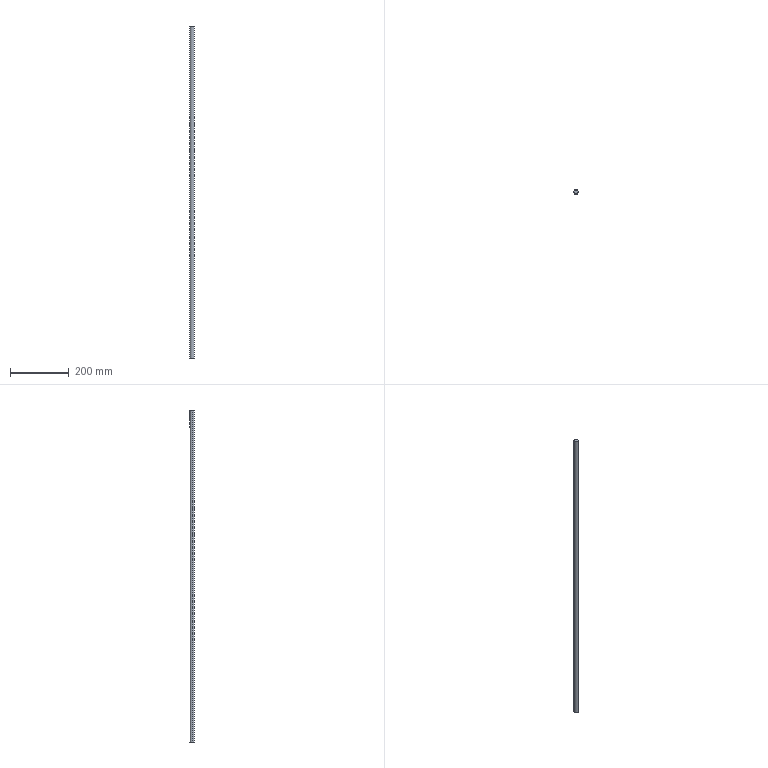Part | SolidWorks | features ICE 3, Extrusion 1 | 1 solid | 14 faces | box 15 x 15 x 1130 mm | volume 199245 mm3 | plane 8 | cylinder 6 | commonest cylinder face diameters 5 x4 15 x2
STEP:
#1=CARTESIAN_POINT('',(0.,7.5,1107.5));
#2=VERTEX_POINT('',#1);
#3=CARTESIAN_POINT('',(2.5,7.071,1110.));
#4=VERTEX_POINT('',#3);
#5=CARTESIAN_POINT('',(0.,7.5,1107.5));
#6=CARTESIAN_POINT('',(0.1643,7.5,1107.5));
#7=CARTESIAN_POINT('',(0.3311,7.494,1107.517));
#8=CARTESIAN_POINT('',(0.6524,7.473,1107.581));
#9=CARTESIAN_POINT('',(0.8088,7.458,1107.629));
#10=CARTESIAN_POINT('',(1.113,7.419,1107.755));
#11=CARTESIAN_POINT('',(1.257,7.395,1107.833));
#12=CARTESIAN_POINT('',(1.526,7.344,1108.013));
#13=CARTESIAN_POINT('',(1.653,7.316,1108.118));
#14=CARTESIAN_POINT('',(1.883,7.261,1108.348));
#15=CARTESIAN_POINT('',(1.986,7.233,1108.473));
#16=CARTESIAN_POINT('',(2.167,7.181,1108.742));
#17=CARTESIAN_POINT('',(2.245,7.156,1108.888));
#18=CARTESIAN_POINT('',(2.37,7.116,1109.189));
#19=CARTESIAN_POINT('',(2.418,7.1,1109.344));
#20=CARTESIAN_POINT('',(2.483,7.077,1109.668));
#21=CARTESIAN_POINT('',(2.5,7.071,1109.834));
#22=CARTESIAN_POINT('',(2.5,7.071,1110.));
#23=B_SPLINE_CURVE_WITH_KNOTS('',3,(#5,#6,#7,#8,#9,#10,#11,#12,#13,#14,#15,#16,#17,#18,#19,#20,#21,#22),.UNSPECIFIED.,.F.,.F.,(4,2,2,2,2,2,2,2,4),(0.003937,0.004429,0.004921,0.005412,0.005904,0.006395,0.006887,0.007378,0.00787),.UNSPECIFIED.);
#24=EDGE_CURVE('',#2,#4,#23,.T.);
#25=ORIENTED_EDGE('',*,*,#24,.F.);
#26=CARTESIAN_POINT('',(0.,4.5,1107.5));
#27=VERTEX_POINT('',#26);
#28=CARTESIAN_POINT('',(0.,7.501,1107.5));
#29=DIRECTION('',(0.,-1.,0.));
#30=VECTOR('',#29,1000.);
#31=LINE('',#28,#30);
#32=EDGE_CURVE('',#2,#27,#31,.T.);
#33=ORIENTED_EDGE('',*,*,#32,.T.);
#34=CARTESIAN_POINT('',(2.5,4.5,1110.));
#35=VERTEX_POINT('',#34);
#36=CARTESIAN_POINT('',(0.,4.5,1110.));
#37=DIRECTION('',(0.,1.,0.));
#38=DIRECTION('',(0.,0.,-1.));
#39=AXIS2_PLACEMENT_3D('',#36,#37,#38);
#40=CIRCLE('',#39,2.5);
#41=EDGE_CURVE('',#35,#27,#40,.T.);
#42=ORIENTED_EDGE('',*,*,#41,.F.);
#43=CARTESIAN_POINT('',(2.5,7.071,1110.));
#44=DIRECTION('',(0.,1.,0.));
#45=VECTOR('',#44,1000.);
#46=LINE('',#43,#45);
#47=EDGE_CURVE('',#35,#4,#46,.T.);
#48=ORIENTED_EDGE('',*,*,#47,.T.);
#49=EDGE_LOOP('',(#25,#33,#42,#48));
#50=FACE_OUTER_BOUND('',#49,.T.);
#51=CARTESIAN_POINT('',(0.,7.501,1110.));
#52=DIRECTION('',(0.,-1.,0.));
#53=DIRECTION('',(0.,0.,-1.));
#54=AXIS2_PLACEMENT_3D('',#51,#52,#53);
#55=CYLINDRICAL_SURFACE('',#54,2.5);
#56=ADVANCED_FACE('',(#50),#55,.F.);
#57=CARTESIAN_POINT('',(-2.5,7.071,1079.079));
#58=VERTEX_POINT('',#57);
#59=CARTESIAN_POINT('',(2.5,7.071,1079.079));
#60=VERTEX_POINT('',#59);
#61=CARTESIAN_POINT('',(-2.5,7.071,1079.079));
#62=CARTESIAN_POINT('',(-2.5,7.071,1079.245));
#63=CARTESIAN_POINT('',(-2.484,7.077,1079.409));
#64=CARTESIAN_POINT('',(-2.419,7.099,1079.73));
#65=CARTESIAN_POINT('',(-2.371,7.116,1079.889));
#66=CARTESIAN_POINT('',(-2.245,7.156,1080.191));
#67=CARTESIAN_POINT('',(-2.168,7.18,1080.334));
#68=CARTESIAN_POINT('',(-1.987,7.233,1080.605));
#69=CARTESIAN_POINT('',(-1.882,7.261,1080.732));
#70=CARTESIAN_POINT('',(-1.539,7.344,1081.075));
#71=CARTESIAN_POINT('',(-1.262,7.399,1081.261));
#72=CARTESIAN_POINT('',(-0.812,7.457,1081.449));
#73=CARTESIAN_POINT('',(-0.6532,7.473,1081.498));
#74=CARTESIAN_POINT('',(-0.33,7.494,1081.563));
#75=CARTESIAN_POINT('',(-0.167,7.5,1081.579));
#76=CARTESIAN_POINT('',(0.1617,7.5,1081.579));
#77=CARTESIAN_POINT('',(0.3287,7.495,1081.563));
#78=CARTESIAN_POINT('',(0.6503,7.473,1081.499));
#79=CARTESIAN_POINT('',(0.8068,7.458,1081.451));
#80=CARTESIAN_POINT('',(1.111,7.419,1081.325));
#81=CARTESIAN_POINT('',(1.255,7.395,1081.247));
#82=CARTESIAN_POINT('',(1.525,7.345,1081.067));
#83=CARTESIAN_POINT('',(1.652,7.317,1080.962));
#84=CARTESIAN_POINT('',(1.882,7.261,1080.732));
#85=CARTESIAN_POINT('',(1.985,7.233,1080.607));
#86=CARTESIAN_POINT('',(2.166,7.181,1080.338));
#87=CARTESIAN_POINT('',(2.245,7.156,1080.192));
#88=CARTESIAN_POINT('',(2.37,7.116,1079.891));
#89=CARTESIAN_POINT('',(2.418,7.1,1079.735));
#90=CARTESIAN_POINT('',(2.483,7.077,1079.412));
#91=CARTESIAN_POINT('',(2.5,7.071,1079.245));
#92=CARTESIAN_POINT('',(2.5,7.071,1079.079));
#93=B_SPLINE_CURVE_WITH_KNOTS('',3,(#61,#62,#63,#64,#65,#66,#67,#68,#69,#70,#71,#72,#73,#74,#75,#76,#77,#78,#79,#80,#81,#82,#83,#84,#85,#86,#87,#88,#89,#90,#91,#92),.UNSPECIFIED.,.F.,.F.,(4,2,2,2,2,2,2,2,2,2,2,2,2,2,2,4),(0.,0.0004919,0.0009837,0.001476,0.001967,0.002951,0.003443,0.003935,0.004427,0.004919,0.00541,0.005902,0.006394,0.006886,0.007378,0.00787),.UNSPECIFIED.);
#94=EDGE_CURVE('',#58,#60,#93,.T.);
#95=ORIENTED_EDGE('',*,*,#94,.F.);
#96=CARTESIAN_POINT('',(-2.5,7.071,1074.079));
#97=VERTEX_POINT('',#96);
#98=CARTESIAN_POINT('',(-2.5,7.071,1130.));
#99=DIRECTION('',(0.,0.,1.));
#100=VECTOR('',#99,1000.);
#101=LINE('',#98,#100);
#102=EDGE_CURVE('',#97,#58,#101,.T.);
#103=ORIENTED_EDGE('',*,*,#102,.F.);
#104=CARTESIAN_POINT('',(2.5,7.071,1074.079));
#105=VERTEX_POINT('',#104);
#106=CARTESIAN_POINT('',(2.5,7.071,1074.079));
#107=CARTESIAN_POINT('',(2.5,7.071,1073.913));
#108=CARTESIAN_POINT('',(2.484,7.077,1073.749));
#109=CARTESIAN_POINT('',(2.419,7.099,1073.428));
#110=CARTESIAN_POINT('',(2.371,7.116,1073.269));
#111=CARTESIAN_POINT('',(2.245,7.156,1072.967));
#112=CARTESIAN_POINT('',(2.168,7.18,1072.824));
#113=CARTESIAN_POINT('',(1.987,7.233,1072.553));
#114=CARTESIAN_POINT('',(1.882,7.261,1072.426));
#115=CARTESIAN_POINT('',(1.539,7.344,1072.083));
#116=CARTESIAN_POINT('',(1.262,7.399,1071.897));
#117=CARTESIAN_POINT('',(0.812,7.457,1071.709));
#118=CARTESIAN_POINT('',(0.6532,7.473,1071.66));
#119=CARTESIAN_POINT('',(0.33,7.494,1071.595));
#120=CARTESIAN_POINT('',(0.167,7.5,1071.579));
#121=CARTESIAN_POINT('',(-0.1617,7.5,1071.579));
#122=CARTESIAN_POINT('',(-0.3287,7.495,1071.595));
#123=CARTESIAN_POINT('',(-0.6503,7.473,1071.66));
#124=CARTESIAN_POINT('',(-0.8068,7.458,1071.707));
#125=CARTESIAN_POINT('',(-1.111,7.419,1071.833));
#126=CARTESIAN_POINT('',(-1.255,7.395,1071.911));
#127=CARTESIAN_POINT('',(-1.525,7.345,1072.091));
#128=CARTESIAN_POINT('',(-1.652,7.317,1072.196));
#129=CARTESIAN_POINT('',(-1.882,7.261,1072.426));
#130=CARTESIAN_POINT('',(-1.985,7.233,1072.551));
#131=CARTESIAN_POINT('',(-2.166,7.181,1072.82));
#132=CARTESIAN_POINT('',(-2.245,7.156,1072.967));
#133=CARTESIAN_POINT('',(-2.37,7.116,1073.267));
#134=CARTESIAN_POINT('',(-2.418,7.1,1073.423));
#135=CARTESIAN_POINT('',(-2.483,7.077,1073.746));
#136=CARTESIAN_POINT('',(-2.5,7.071,1073.913));
#137=CARTESIAN_POINT('',(-2.5,7.071,1074.079));
#138=B_SPLINE_CURVE_WITH_KNOTS('',3,(#106,#107,#108,#109,#110,#111,#112,#113,#114,#115,#116,#117,#118,#119,#120,#121,#122,#123,#124,#125,#126,#127,#128,#129,#130,#131,#132,#133,#134,#135,#136,#137),.UNSPECIFIED.,.F.,.F.,(4,2,2,2,2,2,2,2,2,2,2,2,2,2,2,4),(0.,0.0004919,0.0009837,0.001476,0.001967,0.002951,0.003443,0.003935,0.004427,0.004919,0.00541,0.005902,0.006394,0.006886,0.007378,0.00787),.UNSPECIFIED.);
#139=EDGE_CURVE('',#105,#97,#138,.T.);
#140=ORIENTED_EDGE('',*,*,#139,.F.);
#141=CARTESIAN_POINT('',(2.5,7.071,1130.));
#142=DIRECTION('',(0.,0.,-1.));
#143=VECTOR('',#142,1000.);
#144=LINE('',#141,#143);
#145=EDGE_CURVE('',#60,#105,#144,.T.);
#146=ORIENTED_EDGE('',*,*,#145,.F.);
#147=EDGE_LOOP('',(#95,#103,#140,#146));
#148=FACE_BOUND('',#147,.T.);
#149=CARTESIAN_POINT('',(7.5,0.,1130.));
#150=VERTEX_POINT('',#149);
#151=CARTESIAN_POINT('',(2.5,7.071,1130.));
#152=VERTEX_POINT('',#151);
#153=CARTESIAN_POINT('',(0.,0.,1130.));
#154=DIRECTION('',(0.,0.,1.));
#155=DIRECTION('',(1.,0.,0.));
#156=AXIS2_PLACEMENT_3D('',#153,#154,#155);
#157=CIRCLE('',#156,7.5);
#158=EDGE_CURVE('',#150,#152,#157,.T.);
#159=ORIENTED_EDGE('',*,*,#158,.F.);
#160=CARTESIAN_POINT('',(7.5,0.,0.));
#161=VERTEX_POINT('',#160);
#162=CARTESIAN_POINT('',(7.5,0.,1130.));
#163=DIRECTION('',(0.,0.,-1.));
#164=VECTOR('',#163,1000.);
#165=LINE('',#162,#164);
#166=EDGE_CURVE('',#150,#161,#165,.T.);
#167=ORIENTED_EDGE('',*,*,#166,.T.);
#168=CARTESIAN_POINT('',(-7.5,0.,0.));
#169=VERTEX_POINT('',#168);
#170=CARTESIAN_POINT('',(0.,0.,0.));
#171=DIRECTION('',(0.,0.,1.));
#172=DIRECTION('',(1.,0.,0.));
#173=AXIS2_PLACEMENT_3D('',#170,#171,#172);
#174=CIRCLE('',#173,7.5);
#175=EDGE_CURVE('',#161,#169,#174,.T.);
#176=ORIENTED_EDGE('',*,*,#175,.T.);
#177=CARTESIAN_POINT('',(-7.5,0.,1130.));
#178=VERTEX_POINT('',#177);
#179=CARTESIAN_POINT('',(-7.5,0.,1130.));
#180=DIRECTION('',(0.,0.,-1.));
#181=VECTOR('',#180,1000.);
#182=LINE('',#179,#181);
#183=EDGE_CURVE('',#178,#169,#182,.T.);
#184=ORIENTED_EDGE('',*,*,#183,.F.);
#185=CARTESIAN_POINT('',(-2.5,7.071,1130.));
#186=VERTEX_POINT('',#185);
#187=CARTESIAN_POINT('',(0.,0.,1130.));
#188=DIRECTION('',(0.,0.,1.));
#189=DIRECTION('',(1.,0.,0.));
#190=AXIS2_PLACEMENT_3D('',#187,#188,#189);
#191=CIRCLE('',#190,7.5);
#192=EDGE_CURVE('',#186,#178,#191,.T.);
#193=ORIENTED_EDGE('',*,*,#192,.F.);
#194=CARTESIAN_POINT('',(-2.5,7.071,1110.));
#195=VERTEX_POINT('',#194);
#196=CARTESIAN_POINT('',(-2.5,7.071,1110.));
#197=DIRECTION('',(0.,0.,1.));
#198=VECTOR('',#197,1000.);
#199=LINE('',#196,#198);
#200=EDGE_CURVE('',#195,#186,#199,.T.);
#201=ORIENTED_EDGE('',*,*,#200,.F.);
#202=CARTESIAN_POINT('',(-2.5,7.071,1110.));
#203=CARTESIAN_POINT('',(-2.5,7.071,1109.833));
#204=CARTESIAN_POINT('',(-2.484,7.077,1109.67));
#205=CARTESIAN_POINT('',(-2.419,7.099,1109.349));
#206=CARTESIAN_POINT('',(-2.371,7.116,1109.189));
#207=CARTESIAN_POINT('',(-2.245,7.157,1108.887));
#208=CARTESIAN_POINT('',(-2.168,7.181,1108.744));
#209=CARTESIAN_POINT('',(-1.986,7.233,1108.473));
#210=CARTESIAN_POINT('',(-1.882,7.261,1108.346));
#211=CARTESIAN_POINT('',(-1.538,7.344,1108.003));
#212=CARTESIAN_POINT('',(-1.261,7.399,1107.817));
#213=CARTESIAN_POINT('',(-0.81,7.458,1107.629));
#214=CARTESIAN_POINT('',(-0.6511,7.473,1107.581));
#215=CARTESIAN_POINT('',(-0.3276,7.495,1107.516));
#216=CARTESIAN_POINT('',(-0.1645,7.5,1107.5));
#217=CARTESIAN_POINT('',(0.,7.5,1107.5));
#218=B_SPLINE_CURVE_WITH_KNOTS('',3,(#202,#203,#204,#205,#206,#207,#208,#209,#210,#211,#212,#213,#214,#215,#216,#217),.UNSPECIFIED.,.F.,.F.,(4,2,2,2,2,2,2,4),(0.,0.0004922,0.0009844,0.001477,0.001969,0.002953,0.003445,0.003937),.UNSPECIFIED.);
#219=EDGE_CURVE('',#195,#2,#218,.T.);
#220=ORIENTED_EDGE('',*,*,#219,.T.);
#221=ORIENTED_EDGE('',*,*,#24,.T.);
#222=CARTESIAN_POINT('',(2.5,7.071,1110.));
#223=DIRECTION('',(0.,0.,1.));
#224=VECTOR('',#223,1000.);
#225=LINE('',#222,#224);
#226=EDGE_CURVE('',#4,#152,#225,.T.);
#227=ORIENTED_EDGE('',*,*,#226,.T.);
#228=EDGE_LOOP('',(#159,#167,#176,#184,#193,#201,#220,#221,#227));
#229=FACE_OUTER_BOUND('',#228,.T.);
#230=CARTESIAN_POINT('',(0.,0.,1130.));
#231=DIRECTION('',(0.,0.,-1.));
#232=DIRECTION('',(-1.,0.,0.));
#233=AXIS2_PLACEMENT_3D('',#230,#231,#232);
#234=CYLINDRICAL_SURFACE('',#233,7.5);
#235=ADVANCED_FACE('',(#148,#229),#234,.T.);
#236=ORIENTED_EDGE('',*,*,#166,.F.);
#237=CARTESIAN_POINT('',(0.,0.,1130.));
#238=DIRECTION('',(0.,0.,1.));
#239=DIRECTION('',(1.,0.,0.));
#240=AXIS2_PLACEMENT_3D('',#237,#238,#239);
#241=CIRCLE('',#240,7.5);
#242=EDGE_CURVE('',#178,#150,#241,.T.);
#243=ORIENTED_EDGE('',*,*,#242,.F.);
#244=ORIENTED_EDGE('',*,*,#183,.T.);
#245=CARTESIAN_POINT('',(0.,0.,0.));
#246=DIRECTION('',(0.,0.,1.));
#247=DIRECTION('',(1.,0.,0.));
#248=AXIS2_PLACEMENT_3D('',#245,#246,#247);
#249=CIRCLE('',#248,7.5);
#250=EDGE_CURVE('',#169,#161,#249,.T.);
#251=ORIENTED_EDGE('',*,*,#250,.T.);
#252=EDGE_LOOP('',(#236,#243,#244,#251));
#253=FACE_OUTER_BOUND('',#252,.T.);
#254=CARTESIAN_POINT('',(0.,0.,1130.));
#255=DIRECTION('',(0.,0.,-1.));
#256=DIRECTION('',(-1.,0.,0.));
#257=AXIS2_PLACEMENT_3D('',#254,#255,#256);
#258=CYLINDRICAL_SURFACE('',#257,7.5);
#259=ADVANCED_FACE('',(#253),#258,.T.);
#260=CARTESIAN_POINT('',(2.5,4.5,1130.));
#261=VERTEX_POINT('',#260);
#262=CARTESIAN_POINT('',(2.5,7.071,1130.));
#263=DIRECTION('',(0.,1.,0.));
#264=VECTOR('',#263,1000.);
#265=LINE('',#262,#264);
#266=EDGE_CURVE('',#261,#152,#265,.T.);
#267=ORIENTED_EDGE('',*,*,#266,.F.);
#268=CARTESIAN_POINT('',(-2.5,4.5,1130.));
#269=VERTEX_POINT('',#268);
#270=CARTESIAN_POINT('',(-2.5,4.5,1130.));
#271=DIRECTION('',(1.,0.,0.));
#272=VECTOR('',#271,1000.);
#273=LINE('',#270,#272);
#274=EDGE_CURVE('',#269,#261,#273,.T.);
#275=ORIENTED_EDGE('',*,*,#274,.F.);
#276=CARTESIAN_POINT('',(-2.5,7.071,1130.));
#277=DIRECTION('',(0.,-1.,0.));
#278=VECTOR('',#277,1000.);
#279=LINE('',#276,#278);
#280=EDGE_CURVE('',#186,#269,#279,.T.);
#281=ORIENTED_EDGE('',*,*,#280,.F.);
#282=ORIENTED_EDGE('',*,*,#192,.T.);
#283=ORIENTED_EDGE('',*,*,#242,.T.);
#284=ORIENTED_EDGE('',*,*,#158,.T.);
#285=EDGE_LOOP('',(#267,#275,#281,#282,#283,#284));
#286=FACE_OUTER_BOUND('',#285,.T.);
#287=CARTESIAN_POINT('',(0.,0.,1130.));
#288=DIRECTION('',(0.,0.,1.));
#289=DIRECTION('',(1.,0.,0.));
#290=AXIS2_PLACEMENT_3D('',#287,#288,#289);
#291=PLANE('',#290);
#292=ADVANCED_FACE('',(#286),#291,.T.);
#293=ORIENTED_EDGE('',*,*,#250,.F.);
#294=ORIENTED_EDGE('',*,*,#175,.F.);
#295=EDGE_LOOP('',(#293,#294));
#296=FACE_OUTER_BOUND('',#295,.T.);
#297=CARTESIAN_POINT('',(0.,0.,0.));
#298=DIRECTION('',(0.,0.,1.));
#299=DIRECTION('',(1.,0.,0.));
#300=AXIS2_PLACEMENT_3D('',#297,#298,#299);
#301=PLANE('',#300);
#302=ADVANCED_FACE('',(#296),#301,.F.);
#303=ORIENTED_EDGE('',*,*,#266,.T.);
#304=ORIENTED_EDGE('',*,*,#226,.F.);
#305=ORIENTED_EDGE('',*,*,#47,.F.);
#306=CARTESIAN_POINT('',(2.5,4.5,1110.));
#307=DIRECTION('',(0.,0.,1.));
#308=VECTOR('',#307,1000.);
#309=LINE('',#306,#308);
#310=EDGE_CURVE('',#35,#261,#309,.T.);
#311=ORIENTED_EDGE('',*,*,#310,.T.);
#312=EDGE_LOOP('',(#303,#304,#305,#311));
#313=FACE_OUTER_BOUND('',#312,.T.);
#314=CARTESIAN_POINT('',(2.5,7.071,1110.));
#315=DIRECTION('',(1.,0.,0.));
#316=DIRECTION('',(0.,1.,0.));
#317=AXIS2_PLACEMENT_3D('',#314,#315,#316);
#318=PLANE('',#317);
#319=ADVANCED_FACE('',(#313),#318,.F.);
#320=ORIENTED_EDGE('',*,*,#274,.T.);
#321=ORIENTED_EDGE('',*,*,#310,.F.);
#322=ORIENTED_EDGE('',*,*,#41,.T.);
#323=CARTESIAN_POINT('',(-2.5,4.5,1110.));
#324=VERTEX_POINT('',#323);
#325=CARTESIAN_POINT('',(0.,4.5,1110.));
#326=DIRECTION('',(0.,1.,0.));
#327=DIRECTION('',(0.,0.,-1.));
#328=AXIS2_PLACEMENT_3D('',#325,#326,#327);
#329=CIRCLE('',#328,2.5);
#330=EDGE_CURVE('',#27,#324,#329,.T.);
#331=ORIENTED_EDGE('',*,*,#330,.T.);
#332=CARTESIAN_POINT('',(-2.5,4.5,1110.));
#333=DIRECTION('',(0.,0.,1.));
#334=VECTOR('',#333,1000.);
#335=LINE('',#332,#334);
#336=EDGE_CURVE('',#324,#269,#335,.T.);
#337=ORIENTED_EDGE('',*,*,#336,.T.);
#338=EDGE_LOOP('',(#320,#321,#322,#331,#337));
#339=FACE_OUTER_BOUND('',#338,.T.);
#340=CARTESIAN_POINT('',(-2.5,4.5,1110.));
#341=DIRECTION('',(0.,-1.,0.));
#342=DIRECTION('',(1.,0.,0.));
#343=AXIS2_PLACEMENT_3D('',#340,#341,#342);
#344=PLANE('',#343);
#345=ADVANCED_FACE('',(#339),#344,.F.);
#346=ORIENTED_EDGE('',*,*,#280,.T.);
#347=ORIENTED_EDGE('',*,*,#336,.F.);
#348=CARTESIAN_POINT('',(-2.5,7.071,1110.));
#349=DIRECTION('',(0.,-1.,0.));
#350=VECTOR('',#349,1000.);
#351=LINE('',#348,#350);
#352=EDGE_CURVE('',#195,#324,#351,.T.);
#353=ORIENTED_EDGE('',*,*,#352,.F.);
#354=ORIENTED_EDGE('',*,*,#200,.T.);
#355=EDGE_LOOP('',(#346,#347,#353,#354));
#356=FACE_OUTER_BOUND('',#355,.T.);
#357=CARTESIAN_POINT('',(-2.5,7.071,1110.));
#358=DIRECTION('',(-1.,0.,0.));
#359=DIRECTION('',(0.,-1.,0.));
#360=AXIS2_PLACEMENT_3D('',#357,#358,#359);
#361=PLANE('',#360);
#362=ADVANCED_FACE('',(#356),#361,.F.);
#363=ORIENTED_EDGE('',*,*,#32,.F.);
#364=ORIENTED_EDGE('',*,*,#219,.F.);
#365=ORIENTED_EDGE('',*,*,#352,.T.);
#366=ORIENTED_EDGE('',*,*,#330,.F.);
#367=EDGE_LOOP('',(#363,#364,#365,#366));
#368=FACE_OUTER_BOUND('',#367,.T.);
#369=CARTESIAN_POINT('',(0.,7.501,1110.));
#370=DIRECTION('',(0.,-1.,0.));
#371=DIRECTION('',(0.,0.,-1.));
#372=AXIS2_PLACEMENT_3D('',#369,#370,#371);
#373=CYLINDRICAL_SURFACE('',#372,2.5);
#374=ADVANCED_FACE('',(#368),#373,.F.);
#375=ORIENTED_EDGE('',*,*,#94,.T.);
#376=CARTESIAN_POINT('',(2.5,4.5,1079.079));
#377=VERTEX_POINT('',#376);
#378=CARTESIAN_POINT('',(2.5,21.5,1079.079));
#379=DIRECTION('',(0.,-1.,0.));
#380=VECTOR('',#379,1000.);
#381=LINE('',#378,#380);
#382=EDGE_CURVE('',#60,#377,#381,.T.);
#383=ORIENTED_EDGE('',*,*,#382,.T.);
#384=CARTESIAN_POINT('',(-2.5,4.5,1079.079));
#385=VERTEX_POINT('',#384);
#386=CARTESIAN_POINT('',(0.,4.5,1079.079));
#387=DIRECTION('',(0.,1.,0.));
#388=DIRECTION('',(-1.,0.,0.));
#389=AXIS2_PLACEMENT_3D('',#386,#387,#388);
#390=CIRCLE('',#389,2.5);
#391=EDGE_CURVE('',#385,#377,#390,.T.);
#392=ORIENTED_EDGE('',*,*,#391,.F.);
#393=CARTESIAN_POINT('',(-2.5,21.5,1079.079));
#394=DIRECTION('',(0.,-1.,0.));
#395=VECTOR('',#394,1000.);
#396=LINE('',#393,#395);
#397=EDGE_CURVE('',#58,#385,#396,.T.);
#398=ORIENTED_EDGE('',*,*,#397,.F.);
#399=EDGE_LOOP('',(#375,#383,#392,#398));
#400=FACE_OUTER_BOUND('',#399,.T.);
#401=CARTESIAN_POINT('',(0.,21.5,1079.079));
#402=DIRECTION('',(0.,-1.,0.));
#403=DIRECTION('',(1.,0.,0.));
#404=AXIS2_PLACEMENT_3D('',#401,#402,#403);
#405=CYLINDRICAL_SURFACE('',#404,2.5);
#406=ADVANCED_FACE('',(#400),#405,.F.);
#407=ORIENTED_EDGE('',*,*,#145,.T.);
#408=CARTESIAN_POINT('',(2.5,4.5,1074.079));
#409=VERTEX_POINT('',#408);
#410=CARTESIAN_POINT('',(2.5,21.5,1074.079));
#411=DIRECTION('',(0.,-1.,0.));
#412=VECTOR('',#411,1000.);
#413=LINE('',#410,#412);
#414=EDGE_CURVE('',#105,#409,#413,.T.);
#415=ORIENTED_EDGE('',*,*,#414,.T.);
#416=CARTESIAN_POINT('',(2.5,4.5,1079.079));
#417=DIRECTION('',(0.,0.,-1.));
#418=VECTOR('',#417,1000.);
#419=LINE('',#416,#418);
#420=EDGE_CURVE('',#377,#409,#419,.T.);
#421=ORIENTED_EDGE('',*,*,#420,.F.);
#422=ORIENTED_EDGE('',*,*,#382,.F.);
#423=EDGE_LOOP('',(#407,#415,#421,#422));
#424=FACE_OUTER_BOUND('',#423,.T.);
#425=CARTESIAN_POINT('',(2.5,21.5,1079.079));
#426=DIRECTION('',(-1.,0.,0.));
#427=DIRECTION('',(0.,-1.,0.));
#428=AXIS2_PLACEMENT_3D('',#425,#426,#427);
#429=PLANE('',#428);
#430=ADVANCED_FACE('',(#424),#429,.T.);
#431=ORIENTED_EDGE('',*,*,#139,.T.);
#432=CARTESIAN_POINT('',(-2.5,4.5,1074.079));
#433=VERTEX_POINT('',#432);
#434=CARTESIAN_POINT('',(-2.5,21.5,1074.079));
#435=DIRECTION('',(0.,-1.,0.));
#436=VECTOR('',#435,1000.);
#437=LINE('',#434,#436);
#438=EDGE_CURVE('',#97,#433,#437,.T.);
#439=ORIENTED_EDGE('',*,*,#438,.T.);
#440=CARTESIAN_POINT('',(0.,4.5,1074.079));
#441=DIRECTION('',(0.,1.,0.));
#442=DIRECTION('',(-1.,0.,0.));
#443=AXIS2_PLACEMENT_3D('',#440,#441,#442);
#444=CIRCLE('',#443,2.5);
#445=EDGE_CURVE('',#409,#433,#444,.T.);
#446=ORIENTED_EDGE('',*,*,#445,.F.);
#447=ORIENTED_EDGE('',*,*,#414,.F.);
#448=EDGE_LOOP('',(#431,#439,#446,#447));
#449=FACE_OUTER_BOUND('',#448,.T.);
#450=CARTESIAN_POINT('',(0.,21.5,1074.079));
#451=DIRECTION('',(0.,-1.,0.));
#452=DIRECTION('',(1.,0.,0.));
#453=AXIS2_PLACEMENT_3D('',#450,#451,#452);
#454=CYLINDRICAL_SURFACE('',#453,2.5);
#455=ADVANCED_FACE('',(#449),#454,.F.);
#456=ORIENTED_EDGE('',*,*,#102,.T.);
#457=ORIENTED_EDGE('',*,*,#397,.T.);
#458=CARTESIAN_POINT('',(-2.5,4.5,1079.079));
#459=DIRECTION('',(0.,0.,1.));
#460=VECTOR('',#459,1000.);
#461=LINE('',#458,#460);
#462=EDGE_CURVE('',#433,#385,#461,.T.);
#463=ORIENTED_EDGE('',*,*,#462,.F.);
#464=ORIENTED_EDGE('',*,*,#438,.F.);
#465=EDGE_LOOP('',(#456,#457,#463,#464));
#466=FACE_OUTER_BOUND('',#465,.T.);
#467=CARTESIAN_POINT('',(-2.5,21.5,1079.079));
#468=DIRECTION('',(1.,0.,0.));
#469=DIRECTION('',(0.,1.,0.));
#470=AXIS2_PLACEMENT_3D('',#467,#468,#469);
#471=PLANE('',#470);
#472=ADVANCED_FACE('',(#466),#471,.T.);
#473=ORIENTED_EDGE('',*,*,#391,.T.);
#474=ORIENTED_EDGE('',*,*,#420,.T.);
#475=ORIENTED_EDGE('',*,*,#445,.T.);
#476=ORIENTED_EDGE('',*,*,#462,.T.);
#477=EDGE_LOOP('',(#473,#474,#475,#476));
#478=FACE_OUTER_BOUND('',#477,.T.);
#479=CARTESIAN_POINT('',(0.,4.5,1079.079));
#480=DIRECTION('',(0.,1.,0.));
#481=DIRECTION('',(-1.,0.,0.));
#482=AXIS2_PLACEMENT_3D('',#479,#480,#481);
#483=PLANE('',#482);
#484=ADVANCED_FACE('',(#478),#483,.T.);
#485=CLOSED_SHELL('',(#56,#235,#259,#292,#302,#319,#345,#362,#374,#406,#430,#455,#472,#484));
#486=MANIFOLD_SOLID_BREP('',#485);
#487=CARTESIAN_POINT('',(0.,0.,0.));
#488=DIRECTION('',(0.,0.,1.));
#489=DIRECTION('',(1.,0.,0.));
#490=AXIS2_PLACEMENT_3D('',#487,#488,#489);
#491=(LENGTH_UNIT()NAMED_UNIT(*)SI_UNIT(.MILLI.,.METRE.));
#492=UNCERTAINTY_MEASURE_WITH_UNIT(LENGTH_MEASURE(0.00001),#491,'','');
#493=(NAMED_UNIT(*)PLANE_ANGLE_UNIT()SI_UNIT($,.RADIAN.));
#494=(NAMED_UNIT(*)SI_UNIT($,.STERADIAN.)SOLID_ANGLE_UNIT());
#495=(GEOMETRIC_REPRESENTATION_CONTEXT(3)GLOBAL_UNCERTAINTY_ASSIGNED_CONTEXT((#492))GLOBAL_UNIT_ASSIGNED_CONTEXT((#491,#493,#494))REPRESENTATION_CONTEXT('',''));
#496=ADVANCED_BREP_SHAPE_REPRESENTATION('',(#486,#490),#495);